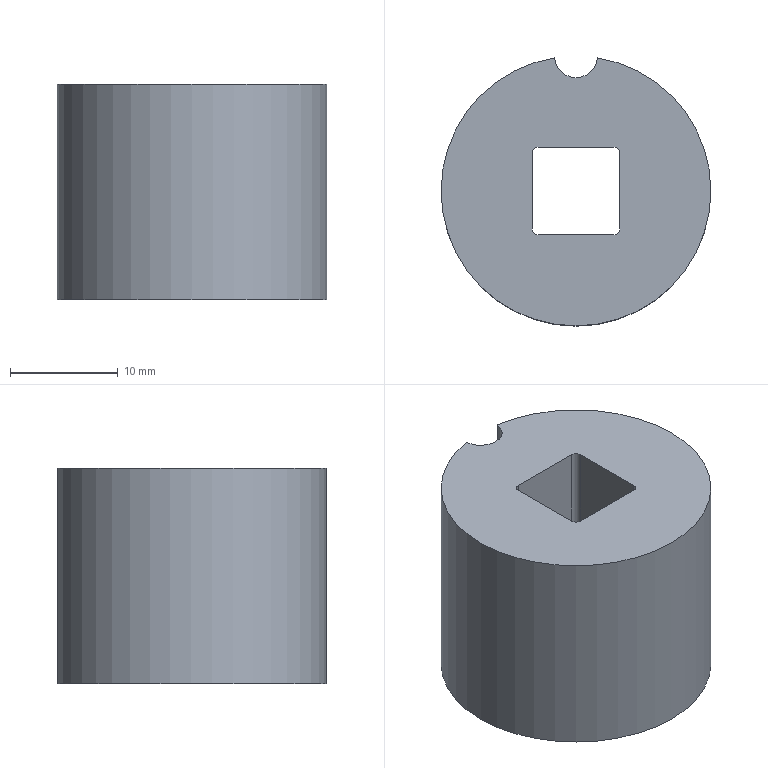Part | NX | features solid 2 | 1 solid | 14 faces | box 25 x 24.84 x 20 mm | volume 6576 mm3 | cylinder 7 | plane 7 | commonest cylinder face diameters 1.1 x4 4 x1 16.6 x1 25 x1
STEP:
#1=CARTESIAN_POINT('',(-223.494,53.291,13.076));
#2=VERTEX_POINT('',#1);
#3=CARTESIAN_POINT('',(-223.494,53.291,33.076));
#4=VERTEX_POINT('',#3);
#5=CARTESIAN_POINT('',(-223.494,53.291,23.076));
#6=DIRECTION('',(0.,0.,1.));
#7=VECTOR('',#6,1000.);
#8=LINE('',#5,#7);
#9=EDGE_CURVE('',#2,#4,#8,.T.);
#10=ORIENTED_EDGE('',*,*,#9,.F.);
#11=CARTESIAN_POINT('',(-219.506,53.291,13.076));
#12=VERTEX_POINT('',#11);
#13=CARTESIAN_POINT('',(-221.5,40.951,13.076));
#14=DIRECTION('',(0.,0.,1.));
#15=DIRECTION('',(0.,1.,0.));
#16=AXIS2_PLACEMENT_3D('',#13,#14,#15);
#17=CIRCLE('',#16,12.5);
#18=EDGE_CURVE('',#2,#12,#17,.T.);
#19=ORIENTED_EDGE('',*,*,#18,.T.);
#20=CARTESIAN_POINT('',(-219.506,53.291,33.076));
#21=VERTEX_POINT('',#20);
#22=CARTESIAN_POINT('',(-219.506,53.291,23.076));
#23=DIRECTION('',(0.,0.,1.));
#24=VECTOR('',#23,1000.);
#25=LINE('',#22,#24);
#26=EDGE_CURVE('',#21,#12,#25,.F.);
#27=ORIENTED_EDGE('',*,*,#26,.F.);
#28=CARTESIAN_POINT('',(-221.5,40.951,33.076));
#29=DIRECTION('',(0.,0.,1.));
#30=DIRECTION('',(0.,1.,0.));
#31=AXIS2_PLACEMENT_3D('',#28,#29,#30);
#32=CIRCLE('',#31,12.5);
#33=EDGE_CURVE('',#4,#21,#32,.T.);
#34=ORIENTED_EDGE('',*,*,#33,.F.);
#35=EDGE_LOOP('',(#10,#19,#27,#34));
#36=FACE_BOUND('',#35,.T.);
#37=CARTESIAN_POINT('',(-221.5,40.951,13.076));
#38=DIRECTION('',(0.,0.,1.));
#39=DIRECTION('',(0.,1.,0.));
#40=AXIS2_PLACEMENT_3D('',#37,#38,#39);
#41=CYLINDRICAL_SURFACE('',#40,12.5);
#42=ADVANCED_FACE('',(#36),#41,.T.);
#43=CARTESIAN_POINT('',(-221.5,49.251,13.076));
#44=VERTEX_POINT('',#43);
#45=CARTESIAN_POINT('',(-221.5,40.951,13.076));
#46=DIRECTION('',(0.,0.,1.));
#47=DIRECTION('',(0.,1.,0.));
#48=AXIS2_PLACEMENT_3D('',#45,#46,#47);
#49=CIRCLE('',#48,8.3);
#50=EDGE_CURVE('',#44,#44,#49,.T.);
#51=ORIENTED_EDGE('',*,*,#50,.T.);
#52=EDGE_LOOP('',(#51));
#53=FACE_BOUND('',#52,.T.);
#54=ORIENTED_EDGE('',*,*,#18,.F.);
#55=CARTESIAN_POINT('',(-221.5,53.451,13.076));
#56=DIRECTION('',(0.,0.,1.));
#57=DIRECTION('',(0.,1.,0.));
#58=AXIS2_PLACEMENT_3D('',#55,#56,#57);
#59=CIRCLE('',#58,2.);
#60=EDGE_CURVE('',#2,#12,#59,.T.);
#61=ORIENTED_EDGE('',*,*,#60,.T.);
#62=EDGE_LOOP('',(#54,#61));
#63=FACE_BOUND('',#62,.T.);
#64=CARTESIAN_POINT('',(-221.5,40.951,13.076));
#65=DIRECTION('',(0.,0.,1.));
#66=DIRECTION('',(0.,1.,0.));
#67=AXIS2_PLACEMENT_3D('',#64,#65,#66);
#68=PLANE('',#67);
#69=ADVANCED_FACE('',(#53,#63),#68,.F.);
#70=CARTESIAN_POINT('',(-225.,36.901,33.076));
#71=VERTEX_POINT('',#70);
#72=CARTESIAN_POINT('',(-218.,36.901,33.076));
#73=VERTEX_POINT('',#72);
#74=CARTESIAN_POINT('',(-225.55,36.901,33.076));
#75=DIRECTION('',(1.,0.,0.));
#76=VECTOR('',#75,1000.);
#77=LINE('',#74,#76);
#78=EDGE_CURVE('',#71,#73,#77,.T.);
#79=ORIENTED_EDGE('',*,*,#78,.F.);
#80=CARTESIAN_POINT('',(-225.55,37.451,33.076));
#81=VERTEX_POINT('',#80);
#82=CARTESIAN_POINT('',(-225.,37.451,33.076));
#83=DIRECTION('',(0.,0.,1.));
#84=DIRECTION('',(0.,1.,0.));
#85=AXIS2_PLACEMENT_3D('',#82,#83,#84);
#86=CIRCLE('',#85,0.55);
#87=EDGE_CURVE('',#71,#81,#86,.F.);
#88=ORIENTED_EDGE('',*,*,#87,.T.);
#89=CARTESIAN_POINT('',(-225.55,44.451,33.076));
#90=VERTEX_POINT('',#89);
#91=CARTESIAN_POINT('',(-225.55,45.001,33.076));
#92=DIRECTION('',(0.,-1.,0.));
#93=VECTOR('',#92,1000.);
#94=LINE('',#91,#93);
#95=EDGE_CURVE('',#90,#81,#94,.T.);
#96=ORIENTED_EDGE('',*,*,#95,.F.);
#97=CARTESIAN_POINT('',(-225.,45.001,33.076));
#98=VERTEX_POINT('',#97);
#99=CARTESIAN_POINT('',(-225.,44.451,33.076));
#100=DIRECTION('',(0.,0.,1.));
#101=DIRECTION('',(0.,1.,0.));
#102=AXIS2_PLACEMENT_3D('',#99,#100,#101);
#103=CIRCLE('',#102,0.55);
#104=EDGE_CURVE('',#90,#98,#103,.F.);
#105=ORIENTED_EDGE('',*,*,#104,.T.);
#106=CARTESIAN_POINT('',(-218.,45.001,33.076));
#107=VERTEX_POINT('',#106);
#108=CARTESIAN_POINT('',(-225.55,45.001,33.076));
#109=DIRECTION('',(1.,0.,0.));
#110=VECTOR('',#109,1000.);
#111=LINE('',#108,#110);
#112=EDGE_CURVE('',#98,#107,#111,.T.);
#113=ORIENTED_EDGE('',*,*,#112,.T.);
#114=CARTESIAN_POINT('',(-217.45,44.451,33.076));
#115=VERTEX_POINT('',#114);
#116=CARTESIAN_POINT('',(-218.,44.451,33.076));
#117=DIRECTION('',(0.,0.,1.));
#118=DIRECTION('',(0.,1.,0.));
#119=AXIS2_PLACEMENT_3D('',#116,#117,#118);
#120=CIRCLE('',#119,0.55);
#121=EDGE_CURVE('',#107,#115,#120,.F.);
#122=ORIENTED_EDGE('',*,*,#121,.T.);
#123=CARTESIAN_POINT('',(-217.45,37.451,33.076));
#124=VERTEX_POINT('',#123);
#125=CARTESIAN_POINT('',(-217.45,36.901,33.076));
#126=DIRECTION('',(0.,1.,0.));
#127=VECTOR('',#126,1000.);
#128=LINE('',#125,#127);
#129=EDGE_CURVE('',#124,#115,#128,.T.);
#130=ORIENTED_EDGE('',*,*,#129,.F.);
#131=CARTESIAN_POINT('',(-218.,37.451,33.076));
#132=DIRECTION('',(0.,0.,1.));
#133=DIRECTION('',(0.,1.,0.));
#134=AXIS2_PLACEMENT_3D('',#131,#132,#133);
#135=CIRCLE('',#134,0.55);
#136=EDGE_CURVE('',#124,#73,#135,.F.);
#137=ORIENTED_EDGE('',*,*,#136,.T.);
#138=EDGE_LOOP('',(#79,#88,#96,#105,#113,#122,#130,#137));
#139=FACE_BOUND('',#138,.T.);
#140=CARTESIAN_POINT('',(-221.5,53.451,33.076));
#141=DIRECTION('',(0.,0.,1.));
#142=DIRECTION('',(0.,1.,0.));
#143=AXIS2_PLACEMENT_3D('',#140,#141,#142);
#144=CIRCLE('',#143,2.);
#145=EDGE_CURVE('',#4,#21,#144,.T.);
#146=ORIENTED_EDGE('',*,*,#145,.F.);
#147=ORIENTED_EDGE('',*,*,#33,.T.);
#148=EDGE_LOOP('',(#146,#147));
#149=FACE_BOUND('',#148,.T.);
#150=CARTESIAN_POINT('',(-221.5,40.951,33.076));
#151=DIRECTION('',(0.,0.,1.));
#152=DIRECTION('',(0.,1.,0.));
#153=AXIS2_PLACEMENT_3D('',#150,#151,#152);
#154=PLANE('',#153);
#155=ADVANCED_FACE('',(#139,#149),#154,.T.);
#156=ORIENTED_EDGE('',*,*,#50,.F.);
#157=EDGE_LOOP('',(#156));
#158=FACE_BOUND('',#157,.T.);
#159=CARTESIAN_POINT('',(-221.5,49.251,25.076));
#160=VERTEX_POINT('',#159);
#161=CARTESIAN_POINT('',(-221.5,40.951,25.076));
#162=DIRECTION('',(0.,0.,1.));
#163=DIRECTION('',(0.,1.,0.));
#164=AXIS2_PLACEMENT_3D('',#161,#162,#163);
#165=CIRCLE('',#164,8.3);
#166=EDGE_CURVE('',#160,#160,#165,.T.);
#167=ORIENTED_EDGE('',*,*,#166,.T.);
#168=EDGE_LOOP('',(#167));
#169=FACE_BOUND('',#168,.T.);
#170=CARTESIAN_POINT('',(-221.5,40.951,13.076));
#171=DIRECTION('',(0.,0.,1.));
#172=DIRECTION('',(0.,1.,0.));
#173=AXIS2_PLACEMENT_3D('',#170,#171,#172);
#174=CYLINDRICAL_SURFACE('',#173,8.3);
#175=ADVANCED_FACE('',(#158,#169),#174,.F.);
#176=CARTESIAN_POINT('',(-225.,45.001,25.076));
#177=VERTEX_POINT('',#176);
#178=CARTESIAN_POINT('',(-218.,45.001,25.076));
#179=VERTEX_POINT('',#178);
#180=CARTESIAN_POINT('',(-221.5,45.001,25.076));
#181=DIRECTION('',(1.,0.,0.));
#182=VECTOR('',#181,1000.);
#183=LINE('',#180,#182);
#184=EDGE_CURVE('',#177,#179,#183,.T.);
#185=ORIENTED_EDGE('',*,*,#184,.F.);
#186=CARTESIAN_POINT('',(-225.55,44.451,25.076));
#187=VERTEX_POINT('',#186);
#188=CARTESIAN_POINT('',(-225.,44.451,25.076));
#189=DIRECTION('',(0.,0.,1.));
#190=DIRECTION('',(0.,1.,0.));
#191=AXIS2_PLACEMENT_3D('',#188,#189,#190);
#192=CIRCLE('',#191,0.55);
#193=EDGE_CURVE('',#177,#187,#192,.T.);
#194=ORIENTED_EDGE('',*,*,#193,.T.);
#195=CARTESIAN_POINT('',(-225.55,37.451,25.076));
#196=VERTEX_POINT('',#195);
#197=CARTESIAN_POINT('',(-225.55,40.951,25.076));
#198=DIRECTION('',(0.,-1.,0.));
#199=VECTOR('',#198,1000.);
#200=LINE('',#197,#199);
#201=EDGE_CURVE('',#187,#196,#200,.T.);
#202=ORIENTED_EDGE('',*,*,#201,.T.);
#203=CARTESIAN_POINT('',(-225.,36.901,25.076));
#204=VERTEX_POINT('',#203);
#205=CARTESIAN_POINT('',(-225.,37.451,25.076));
#206=DIRECTION('',(0.,0.,1.));
#207=DIRECTION('',(0.,1.,0.));
#208=AXIS2_PLACEMENT_3D('',#205,#206,#207);
#209=CIRCLE('',#208,0.55);
#210=EDGE_CURVE('',#196,#204,#209,.T.);
#211=ORIENTED_EDGE('',*,*,#210,.T.);
#212=CARTESIAN_POINT('',(-218.,36.901,25.076));
#213=VERTEX_POINT('',#212);
#214=CARTESIAN_POINT('',(-221.5,36.901,25.076));
#215=DIRECTION('',(1.,0.,0.));
#216=VECTOR('',#215,1000.);
#217=LINE('',#214,#216);
#218=EDGE_CURVE('',#204,#213,#217,.T.);
#219=ORIENTED_EDGE('',*,*,#218,.T.);
#220=CARTESIAN_POINT('',(-217.45,37.451,25.076));
#221=VERTEX_POINT('',#220);
#222=CARTESIAN_POINT('',(-218.,37.451,25.076));
#223=DIRECTION('',(0.,0.,1.));
#224=DIRECTION('',(0.,1.,0.));
#225=AXIS2_PLACEMENT_3D('',#222,#223,#224);
#226=CIRCLE('',#225,0.55);
#227=EDGE_CURVE('',#213,#221,#226,.T.);
#228=ORIENTED_EDGE('',*,*,#227,.T.);
#229=CARTESIAN_POINT('',(-217.45,44.451,25.076));
#230=VERTEX_POINT('',#229);
#231=CARTESIAN_POINT('',(-217.45,40.951,25.076));
#232=DIRECTION('',(0.,1.,0.));
#233=VECTOR('',#232,1000.);
#234=LINE('',#231,#233);
#235=EDGE_CURVE('',#221,#230,#234,.T.);
#236=ORIENTED_EDGE('',*,*,#235,.T.);
#237=CARTESIAN_POINT('',(-218.,44.451,25.076));
#238=DIRECTION('',(0.,0.,1.));
#239=DIRECTION('',(0.,1.,0.));
#240=AXIS2_PLACEMENT_3D('',#237,#238,#239);
#241=CIRCLE('',#240,0.55);
#242=EDGE_CURVE('',#230,#179,#241,.T.);
#243=ORIENTED_EDGE('',*,*,#242,.T.);
#244=EDGE_LOOP('',(#185,#194,#202,#211,#219,#228,#236,#243));
#245=FACE_BOUND('',#244,.T.);
#246=ORIENTED_EDGE('',*,*,#166,.F.);
#247=EDGE_LOOP('',(#246));
#248=FACE_BOUND('',#247,.T.);
#249=CARTESIAN_POINT('',(-221.5,40.951,25.076));
#250=DIRECTION('',(0.,0.,1.));
#251=DIRECTION('',(0.,1.,0.));
#252=AXIS2_PLACEMENT_3D('',#249,#250,#251);
#253=PLANE('',#252);
#254=ADVANCED_FACE('',(#245,#248),#253,.F.);
#255=ORIENTED_EDGE('',*,*,#9,.T.);
#256=ORIENTED_EDGE('',*,*,#145,.T.);
#257=ORIENTED_EDGE('',*,*,#26,.T.);
#258=ORIENTED_EDGE('',*,*,#60,.F.);
#259=EDGE_LOOP('',(#255,#256,#257,#258));
#260=FACE_BOUND('',#259,.T.);
#261=CARTESIAN_POINT('',(-221.5,53.451,13.076));
#262=DIRECTION('',(0.,0.,1.));
#263=DIRECTION('',(0.,1.,0.));
#264=AXIS2_PLACEMENT_3D('',#261,#262,#263);
#265=CYLINDRICAL_SURFACE('',#264,2.);
#266=ADVANCED_FACE('',(#260),#265,.F.);
#267=ORIENTED_EDGE('',*,*,#78,.T.);
#268=CARTESIAN_POINT('',(-218.,36.901,25.076));
#269=DIRECTION('',(0.,0.,1.));
#270=VECTOR('',#269,1000.);
#271=LINE('',#268,#270);
#272=EDGE_CURVE('',#73,#213,#271,.F.);
#273=ORIENTED_EDGE('',*,*,#272,.T.);
#274=ORIENTED_EDGE('',*,*,#218,.F.);
#275=CARTESIAN_POINT('',(-225.,36.901,33.076));
#276=DIRECTION('',(0.,0.,1.));
#277=VECTOR('',#276,1000.);
#278=LINE('',#275,#277);
#279=EDGE_CURVE('',#204,#71,#278,.T.);
#280=ORIENTED_EDGE('',*,*,#279,.T.);
#281=EDGE_LOOP('',(#267,#273,#274,#280));
#282=FACE_BOUND('',#281,.T.);
#283=CARTESIAN_POINT('',(-225.55,36.901,13.076));
#284=DIRECTION('',(0.,-1.,0.));
#285=DIRECTION('',(0.,0.,1.));
#286=AXIS2_PLACEMENT_3D('',#283,#284,#285);
#287=PLANE('',#286);
#288=ADVANCED_FACE('',(#282),#287,.F.);
#289=ORIENTED_EDGE('',*,*,#129,.T.);
#290=CARTESIAN_POINT('',(-217.45,44.451,13.076));
#291=DIRECTION('',(0.,0.,1.));
#292=VECTOR('',#291,1000.);
#293=LINE('',#290,#292);
#294=EDGE_CURVE('',#115,#230,#293,.F.);
#295=ORIENTED_EDGE('',*,*,#294,.T.);
#296=ORIENTED_EDGE('',*,*,#235,.F.);
#297=CARTESIAN_POINT('',(-217.45,37.451,33.076));
#298=DIRECTION('',(0.,0.,1.));
#299=VECTOR('',#298,1000.);
#300=LINE('',#297,#299);
#301=EDGE_CURVE('',#221,#124,#300,.T.);
#302=ORIENTED_EDGE('',*,*,#301,.T.);
#303=EDGE_LOOP('',(#289,#295,#296,#302));
#304=FACE_BOUND('',#303,.T.);
#305=CARTESIAN_POINT('',(-217.45,36.901,13.076));
#306=DIRECTION('',(1.,0.,0.));
#307=DIRECTION('',(0.,0.,-1.));
#308=AXIS2_PLACEMENT_3D('',#305,#306,#307);
#309=PLANE('',#308);
#310=ADVANCED_FACE('',(#304),#309,.F.);
#311=ORIENTED_EDGE('',*,*,#112,.F.);
#312=CARTESIAN_POINT('',(-225.,45.001,13.076));
#313=DIRECTION('',(0.,0.,1.));
#314=VECTOR('',#313,1000.);
#315=LINE('',#312,#314);
#316=EDGE_CURVE('',#98,#177,#315,.F.);
#317=ORIENTED_EDGE('',*,*,#316,.T.);
#318=ORIENTED_EDGE('',*,*,#184,.T.);
#319=CARTESIAN_POINT('',(-218.,45.001,13.076));
#320=DIRECTION('',(0.,0.,1.));
#321=VECTOR('',#320,1000.);
#322=LINE('',#319,#321);
#323=EDGE_CURVE('',#179,#107,#322,.T.);
#324=ORIENTED_EDGE('',*,*,#323,.T.);
#325=EDGE_LOOP('',(#311,#317,#318,#324));
#326=FACE_BOUND('',#325,.T.);
#327=CARTESIAN_POINT('',(-225.55,45.001,13.076));
#328=DIRECTION('',(0.,-1.,0.));
#329=DIRECTION('',(0.,0.,1.));
#330=AXIS2_PLACEMENT_3D('',#327,#328,#329);
#331=PLANE('',#330);
#332=ADVANCED_FACE('',(#326),#331,.T.);
#333=ORIENTED_EDGE('',*,*,#201,.F.);
#334=CARTESIAN_POINT('',(-225.55,44.451,13.076));
#335=DIRECTION('',(0.,0.,1.));
#336=VECTOR('',#335,1000.);
#337=LINE('',#334,#336);
#338=EDGE_CURVE('',#187,#90,#337,.T.);
#339=ORIENTED_EDGE('',*,*,#338,.T.);
#340=ORIENTED_EDGE('',*,*,#95,.T.);
#341=CARTESIAN_POINT('',(-225.55,37.451,25.076));
#342=DIRECTION('',(0.,0.,1.));
#343=VECTOR('',#342,1000.);
#344=LINE('',#341,#343);
#345=EDGE_CURVE('',#81,#196,#344,.F.);
#346=ORIENTED_EDGE('',*,*,#345,.T.);
#347=EDGE_LOOP('',(#333,#339,#340,#346));
#348=FACE_BOUND('',#347,.T.);
#349=CARTESIAN_POINT('',(-225.55,45.001,13.076));
#350=DIRECTION('',(-1.,0.,0.));
#351=DIRECTION('',(0.,0.,1.));
#352=AXIS2_PLACEMENT_3D('',#349,#350,#351);
#353=PLANE('',#352);
#354=ADVANCED_FACE('',(#348),#353,.F.);
#355=ORIENTED_EDGE('',*,*,#193,.F.);
#356=ORIENTED_EDGE('',*,*,#316,.F.);
#357=ORIENTED_EDGE('',*,*,#104,.F.);
#358=ORIENTED_EDGE('',*,*,#338,.F.);
#359=EDGE_LOOP('',(#355,#356,#357,#358));
#360=FACE_BOUND('',#359,.T.);
#361=CARTESIAN_POINT('',(-225.,44.451,13.076));
#362=DIRECTION('',(0.,0.,1.));
#363=DIRECTION('',(0.,1.,0.));
#364=AXIS2_PLACEMENT_3D('',#361,#362,#363);
#365=CYLINDRICAL_SURFACE('',#364,0.55);
#366=ADVANCED_FACE('',(#360),#365,.F.);
#367=ORIENTED_EDGE('',*,*,#242,.F.);
#368=ORIENTED_EDGE('',*,*,#294,.F.);
#369=ORIENTED_EDGE('',*,*,#121,.F.);
#370=ORIENTED_EDGE('',*,*,#323,.F.);
#371=EDGE_LOOP('',(#367,#368,#369,#370));
#372=FACE_BOUND('',#371,.T.);
#373=CARTESIAN_POINT('',(-218.,44.451,13.076));
#374=DIRECTION('',(0.,0.,1.));
#375=DIRECTION('',(0.,1.,0.));
#376=AXIS2_PLACEMENT_3D('',#373,#374,#375);
#377=CYLINDRICAL_SURFACE('',#376,0.55);
#378=ADVANCED_FACE('',(#372),#377,.F.);
#379=ORIENTED_EDGE('',*,*,#227,.F.);
#380=ORIENTED_EDGE('',*,*,#272,.F.);
#381=ORIENTED_EDGE('',*,*,#136,.F.);
#382=ORIENTED_EDGE('',*,*,#301,.F.);
#383=EDGE_LOOP('',(#379,#380,#381,#382));
#384=FACE_BOUND('',#383,.T.);
#385=CARTESIAN_POINT('',(-218.,37.451,13.076));
#386=DIRECTION('',(0.,0.,-1.));
#387=DIRECTION('',(0.,-1.,0.));
#388=AXIS2_PLACEMENT_3D('',#385,#386,#387);
#389=CYLINDRICAL_SURFACE('',#388,0.55);
#390=ADVANCED_FACE('',(#384),#389,.F.);
#391=ORIENTED_EDGE('',*,*,#210,.F.);
#392=ORIENTED_EDGE('',*,*,#345,.F.);
#393=ORIENTED_EDGE('',*,*,#87,.F.);
#394=ORIENTED_EDGE('',*,*,#279,.F.);
#395=EDGE_LOOP('',(#391,#392,#393,#394));
#396=FACE_BOUND('',#395,.T.);
#397=CARTESIAN_POINT('',(-225.,37.451,13.076));
#398=DIRECTION('',(0.,0.,-1.));
#399=DIRECTION('',(0.,-1.,0.));
#400=AXIS2_PLACEMENT_3D('',#397,#398,#399);
#401=CYLINDRICAL_SURFACE('',#400,0.55);
#402=ADVANCED_FACE('',(#396),#401,.F.);
#403=CLOSED_SHELL('',(#42,#69,#155,#175,#254,#266,#288,#310,#332,#354,#366,#378,#390,#402));
#404=MANIFOLD_SOLID_BREP('',#403);
#405=(LENGTH_UNIT()NAMED_UNIT(*)SI_UNIT(.MILLI.,.METRE.));
#406=UNCERTAINTY_MEASURE_WITH_UNIT(LENGTH_MEASURE(0.00001),#405,'','');
#407=(NAMED_UNIT(*)PLANE_ANGLE_UNIT()SI_UNIT($,.RADIAN.));
#408=(NAMED_UNIT(*)SI_UNIT($,.STERADIAN.)SOLID_ANGLE_UNIT());
#409=(GEOMETRIC_REPRESENTATION_CONTEXT(3)GLOBAL_UNCERTAINTY_ASSIGNED_CONTEXT((#406))GLOBAL_UNIT_ASSIGNED_CONTEXT((#405,#407,#408))REPRESENTATION_CONTEXT('',''));
#410=ADVANCED_BREP_SHAPE_REPRESENTATION('',(#404),#409);